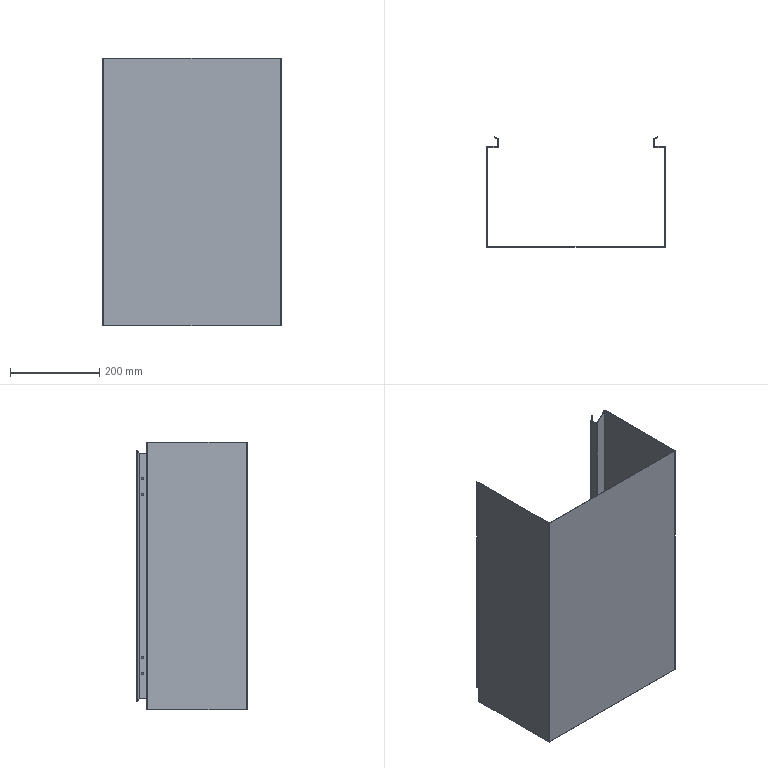Part | SolidWorks | features Cut 4, FlatPattern 1, MirrorSolid 1, SMBaseFlange 1, SheetMetal 1 | 1 solid | 86 faces | box 400 x 247 x 600 mm | volume 843291 mm3 | plane 54 | cylinder 24 | spline 8 | commonest cylinder face diameters 0.6 x8 3.6 x8 5.2 x8